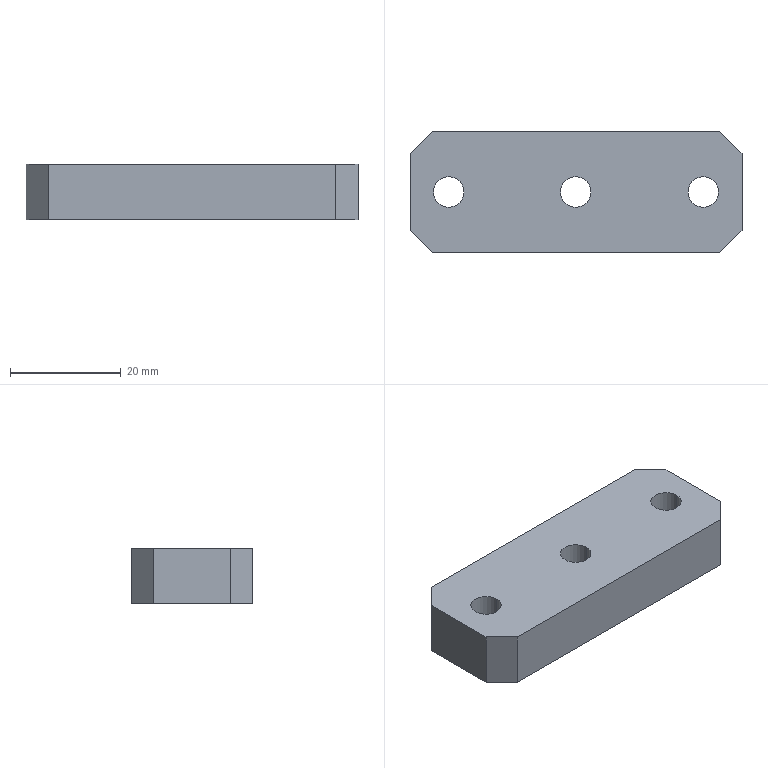Part | Creo | 1 solid | 102 faces | box 60 x 22 x 10 mm | volume 11317 mm3 | other 57 | plane 32 | cylinder 13 | commonest cylinder face diameters 5.5 x6 9.5 x6 45.582 x1